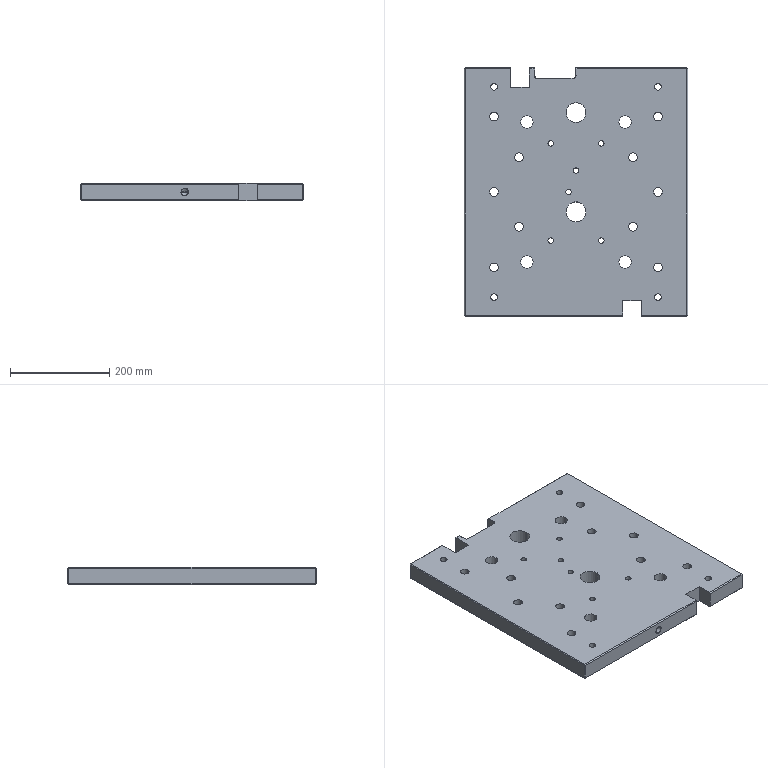Part | Creo | 3 solids | 374 faces | box 450 x 500 x 35 mm | volume 7349704 mm3 | plane 142 | cylinder 118 | other 98 | cone 16 | commonest cylinder face diameters 17.4 x20 25.4 x20 11 x12 17.5 x12 13.4 x8 19.4 x8